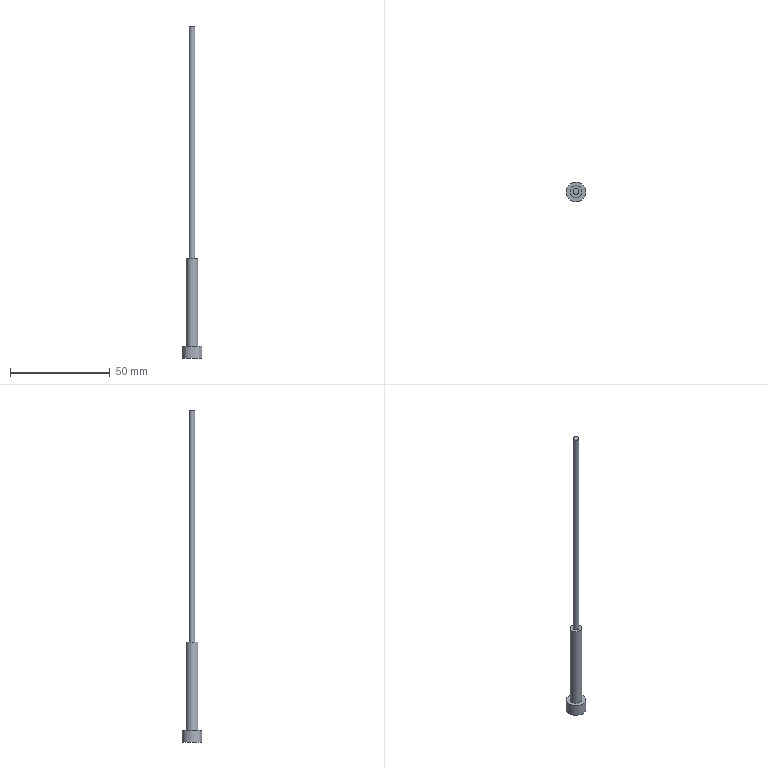Part | STEP file | DDZ6.00_id50_x_t | 1 solid | 7 faces | box 10 x 10 x 166.5 mm | volume 2539 mm3 | plane 4 | cylinder 3 | commonest cylinder face diameters 3 x1 6 x1 10 x1
STEP:
#1=CARTESIAN_POINT('',(-3.,-58.,-129.5));
#2=VERTEX_POINT('',#1);
#3=CARTESIAN_POINT('',(0.,-58.,-129.5));
#4=DIRECTION('',(0.,0.,1.));
#5=DIRECTION('',(-1.,0.,0.));
#6=AXIS2_PLACEMENT_3D('',#3,#4,#5);
#7=CIRCLE('',#6,3.);
#8=EDGE_CURVE('',#2,#2,#7,.T.);
#9=ORIENTED_EDGE('',*,*,#8,.F.);
#10=EDGE_LOOP('',(#9));
#11=FACE_BOUND('',#10,.T.);
#12=CARTESIAN_POINT('',(5.,-58.,-129.5));
#13=VERTEX_POINT('',#12);
#14=CARTESIAN_POINT('',(0.,-58.,-129.5));
#15=DIRECTION('',(0.,0.,-1.));
#16=DIRECTION('',(1.,0.,0.));
#17=AXIS2_PLACEMENT_3D('',#14,#15,#16);
#18=CIRCLE('',#17,5.);
#19=EDGE_CURVE('',#13,#13,#18,.T.);
#20=ORIENTED_EDGE('',*,*,#19,.F.);
#21=EDGE_LOOP('',(#20));
#22=FACE_BOUND('',#21,.T.);
#23=CARTESIAN_POINT('',(0.,-58.,-129.5));
#24=DIRECTION('',(0.,0.,1.));
#25=DIRECTION('',(-1.,0.,0.));
#26=AXIS2_PLACEMENT_3D('',#23,#24,#25);
#27=PLANE('',#26);
#28=ADVANCED_FACE('',(#11,#22),#27,.T.);
#29=ORIENTED_EDGE('',*,*,#19,.T.);
#30=EDGE_LOOP('',(#29));
#31=FACE_BOUND('',#30,.T.);
#32=CARTESIAN_POINT('',(-5.,-58.,-135.5));
#33=VERTEX_POINT('',#32);
#34=CARTESIAN_POINT('',(0.,-58.,-135.5));
#35=DIRECTION('',(0.,0.,1.));
#36=DIRECTION('',(-1.,0.,0.));
#37=AXIS2_PLACEMENT_3D('',#34,#35,#36);
#38=CIRCLE('',#37,5.);
#39=EDGE_CURVE('',#33,#33,#38,.T.);
#40=ORIENTED_EDGE('',*,*,#39,.T.);
#41=EDGE_LOOP('',(#40));
#42=FACE_BOUND('',#41,.T.);
#43=CARTESIAN_POINT('',(0.,-58.,-135.5));
#44=DIRECTION('',(0.,0.,1.));
#45=DIRECTION('',(-1.,0.,0.));
#46=AXIS2_PLACEMENT_3D('',#43,#44,#45);
#47=CYLINDRICAL_SURFACE('',#46,5.);
#48=ADVANCED_FACE('',(#31,#42),#47,.T.);
#49=ORIENTED_EDGE('',*,*,#39,.F.);
#50=EDGE_LOOP('',(#49));
#51=FACE_OUTER_BOUND('',#50,.T.);
#52=CARTESIAN_POINT('',(0.,-58.,-135.5));
#53=DIRECTION('',(0.,0.,-1.));
#54=DIRECTION('',(1.,0.,0.));
#55=AXIS2_PLACEMENT_3D('',#52,#53,#54);
#56=PLANE('',#55);
#57=ADVANCED_FACE('',(#51),#56,.T.);
#58=CARTESIAN_POINT('',(-3.,-58.,-85.5));
#59=VERTEX_POINT('',#58);
#60=CARTESIAN_POINT('',(0.,-58.,-85.5));
#61=DIRECTION('',(0.,0.,1.));
#62=DIRECTION('',(-1.,0.,0.));
#63=AXIS2_PLACEMENT_3D('',#60,#61,#62);
#64=CIRCLE('',#63,3.);
#65=EDGE_CURVE('',#59,#59,#64,.T.);
#66=ORIENTED_EDGE('',*,*,#65,.F.);
#67=EDGE_LOOP('',(#66));
#68=FACE_BOUND('',#67,.T.);
#69=ORIENTED_EDGE('',*,*,#8,.T.);
#70=EDGE_LOOP('',(#69));
#71=FACE_BOUND('',#70,.T.);
#72=CARTESIAN_POINT('',(0.,-58.,-89.5));
#73=DIRECTION('',(0.,0.,-1.));
#74=DIRECTION('',(1.,0.,0.));
#75=AXIS2_PLACEMENT_3D('',#72,#73,#74);
#76=CYLINDRICAL_SURFACE('',#75,3.);
#77=ADVANCED_FACE('',(#68,#71),#76,.T.);
#78=CARTESIAN_POINT('',(-1.5,-58.,-85.5));
#79=VERTEX_POINT('',#78);
#80=CARTESIAN_POINT('',(0.,-58.,-85.5));
#81=DIRECTION('',(0.,0.,-1.));
#82=DIRECTION('',(-1.,0.,0.));
#83=AXIS2_PLACEMENT_3D('',#80,#81,#82);
#84=CIRCLE('',#83,1.5);
#85=EDGE_CURVE('',#79,#79,#84,.T.);
#86=ORIENTED_EDGE('',*,*,#85,.T.);
#87=EDGE_LOOP('',(#86));
#88=FACE_BOUND('',#87,.T.);
#89=ORIENTED_EDGE('',*,*,#65,.T.);
#90=EDGE_LOOP('',(#89));
#91=FACE_BOUND('',#90,.T.);
#92=CARTESIAN_POINT('',(0.,-58.,-85.5));
#93=DIRECTION('',(0.,0.,1.));
#94=DIRECTION('',(-1.,0.,0.));
#95=AXIS2_PLACEMENT_3D('',#92,#93,#94);
#96=PLANE('',#95);
#97=ADVANCED_FACE('',(#88,#91),#96,.T.);
#98=CARTESIAN_POINT('',(-1.5,-58.,31.));
#99=VERTEX_POINT('',#98);
#100=CARTESIAN_POINT('',(0.,-58.,31.));
#101=DIRECTION('',(0.,0.,-1.));
#102=DIRECTION('',(-1.,0.,0.));
#103=AXIS2_PLACEMENT_3D('',#100,#101,#102);
#104=CIRCLE('',#103,1.5);
#105=EDGE_CURVE('',#99,#99,#104,.T.);
#106=ORIENTED_EDGE('',*,*,#105,.F.);
#107=EDGE_LOOP('',(#106));
#108=FACE_OUTER_BOUND('',#107,.T.);
#109=CARTESIAN_POINT('',(0.,-58.,31.));
#110=DIRECTION('',(0.,0.,1.));
#111=DIRECTION('',(-1.,0.,0.));
#112=AXIS2_PLACEMENT_3D('',#109,#110,#111);
#113=PLANE('',#112);
#114=ADVANCED_FACE('',(#108),#113,.T.);
#115=ORIENTED_EDGE('',*,*,#85,.F.);
#116=EDGE_LOOP('',(#115));
#117=FACE_BOUND('',#116,.T.);
#118=ORIENTED_EDGE('',*,*,#105,.T.);
#119=EDGE_LOOP('',(#118));
#120=FACE_BOUND('',#119,.T.);
#121=CARTESIAN_POINT('',(0.,-58.,-140.5));
#122=DIRECTION('',(0.,0.,1.));
#123=DIRECTION('',(-1.,0.,0.));
#124=AXIS2_PLACEMENT_3D('',#121,#122,#123);
#125=CYLINDRICAL_SURFACE('',#124,1.5);
#126=ADVANCED_FACE('',(#117,#120),#125,.T.);
#127=CLOSED_SHELL('',(#28,#48,#57,#77,#97,#114,#126));
#128=MANIFOLD_SOLID_BREP('',#127);
#129=(LENGTH_UNIT()NAMED_UNIT(*)SI_UNIT(.MILLI.,.METRE.));
#130=UNCERTAINTY_MEASURE_WITH_UNIT(LENGTH_MEASURE(0.00002),#129,'','');
#131=(NAMED_UNIT(*)PLANE_ANGLE_UNIT()SI_UNIT($,.RADIAN.));
#132=PLANE_ANGLE_MEASURE_WITH_UNIT(PLANE_ANGLE_MEASURE(0.01745),#131);
#133=DIMENSIONAL_EXPONENTS(0.,0.,0.,0.,0.,0.,0.);
#134=(CONVERSION_BASED_UNIT('DEGREE',#132)NAMED_UNIT(#133)PLANE_ANGLE_UNIT());
#135=(NAMED_UNIT(*)SI_UNIT($,.STERADIAN.)SOLID_ANGLE_UNIT());
#136=(GEOMETRIC_REPRESENTATION_CONTEXT(3)GLOBAL_UNCERTAINTY_ASSIGNED_CONTEXT((#130))GLOBAL_UNIT_ASSIGNED_CONTEXT((#129,#134,#135))REPRESENTATION_CONTEXT('',''));
#137=ADVANCED_BREP_SHAPE_REPRESENTATION('',(#128),#136);